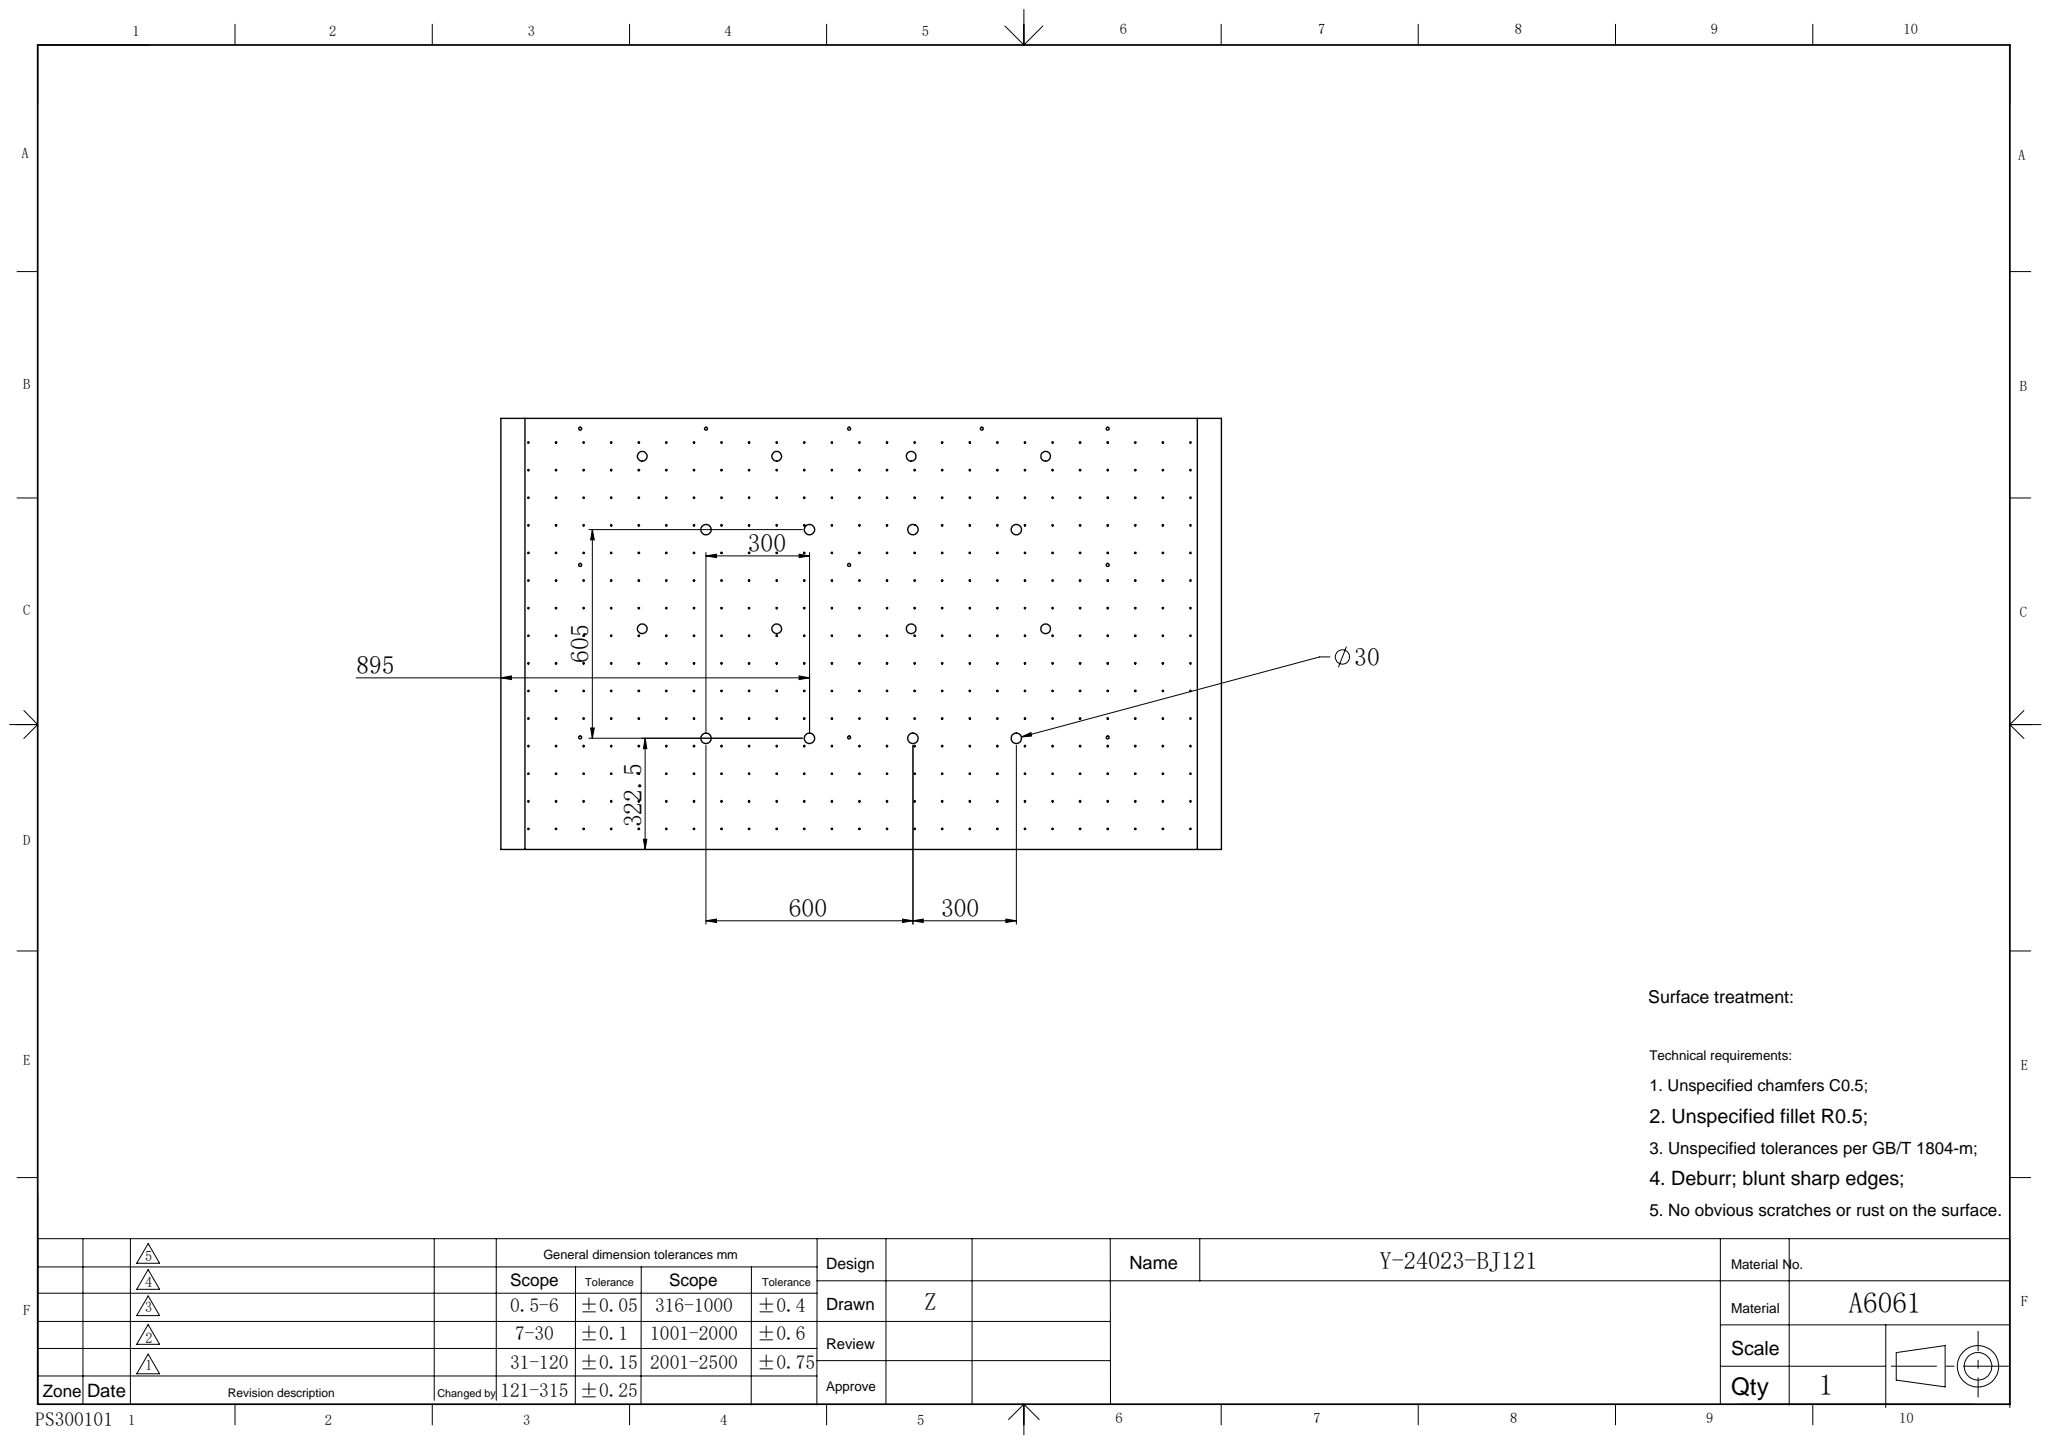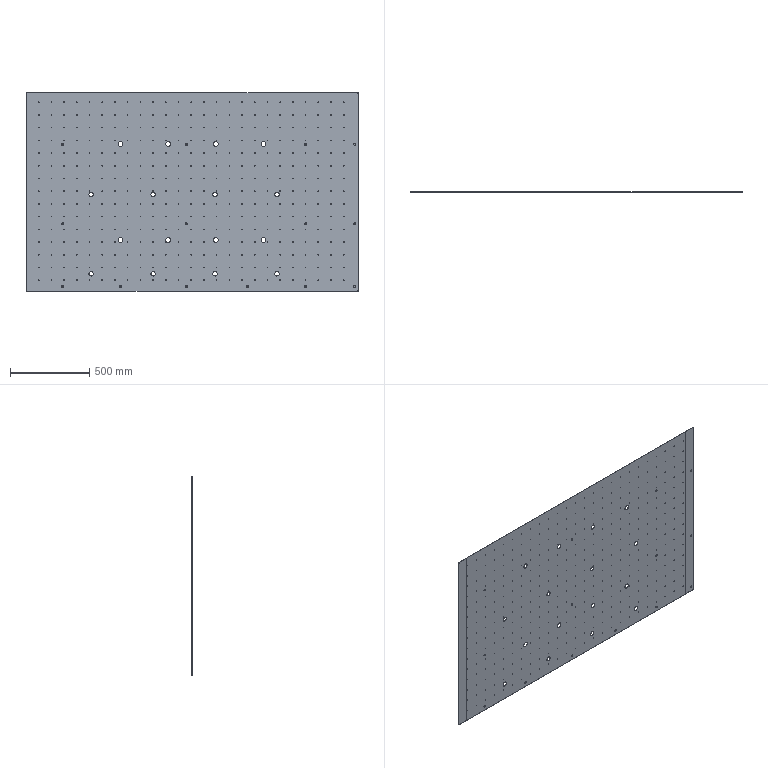Part | SolidWorks | features HoleWzd 3, ICE 3, Fillet 2, Extrusion 1 | 3 solids | 832 faces | box 2090 x 2.5 x 1250 mm | volume 5366829 mm3 | cylinder 786 | cone 28 | plane 18 | commonest cylinder face diameters 4 x749 30 x17 28 x16 10 x2 20 x2